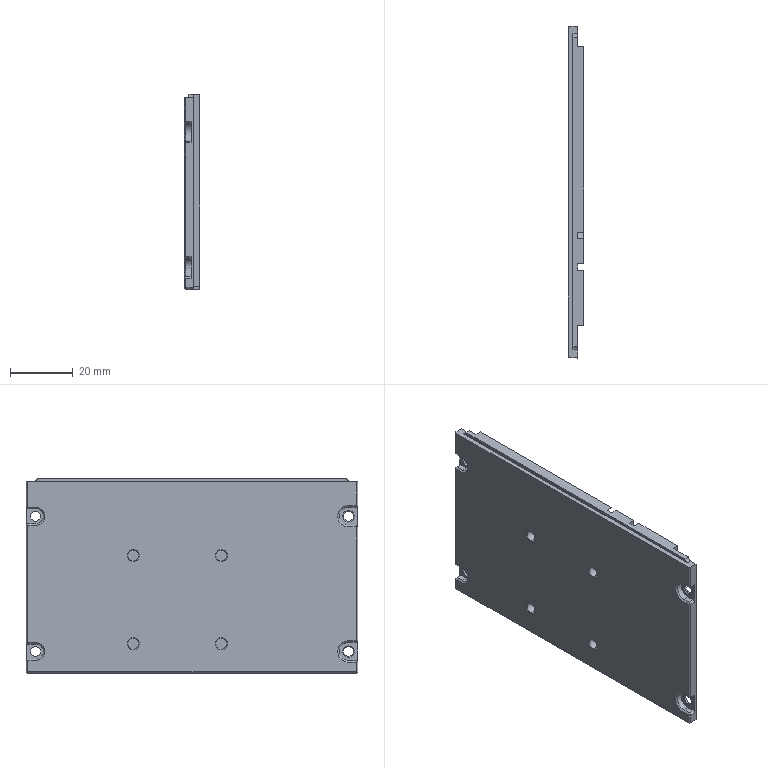Part | SolidWorks | features BaseBody 1 | 1 solid | 120 faces | box 5 x 105.4 x 62 mm | volume 29217 mm3 | plane 74 | cylinder 30 | cone 16 | commonest cylinder face diameters 3.2 x8 3.5 x8 2 x4 6 x4 1.6 x2 4.78 x2